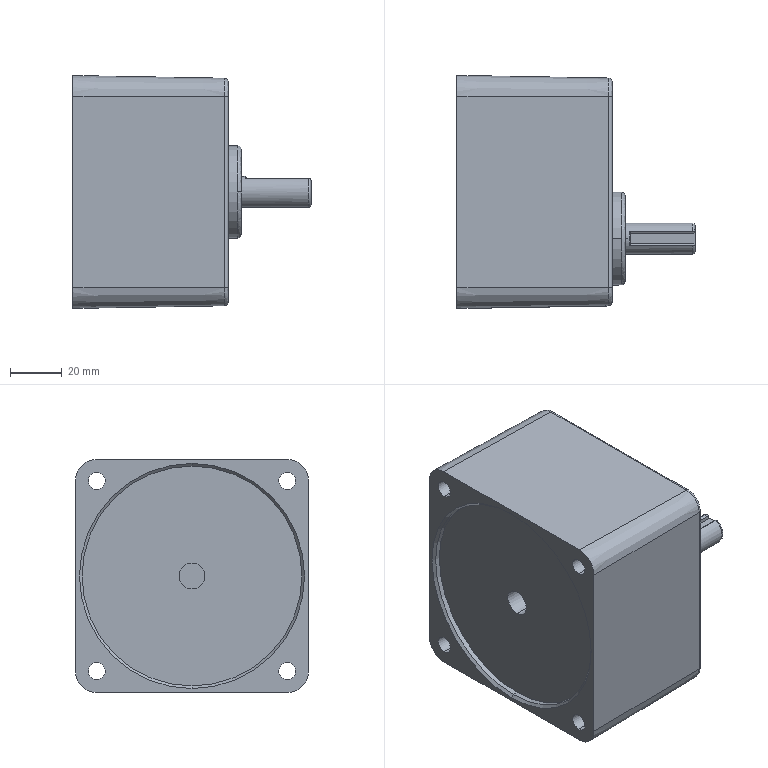Part | STEP file | ADMI9201SOYF_24_1_1 | 1 solid | 77 faces | box 92 x 90 x 90 mm | volume 446981 mm3 | cone 22 | cylinder 20 | plane 20 | spline 15 | commonest cylinder face diameters 6.5 x8 3 x4 10 x2 12 x2 13 x2 85 x2